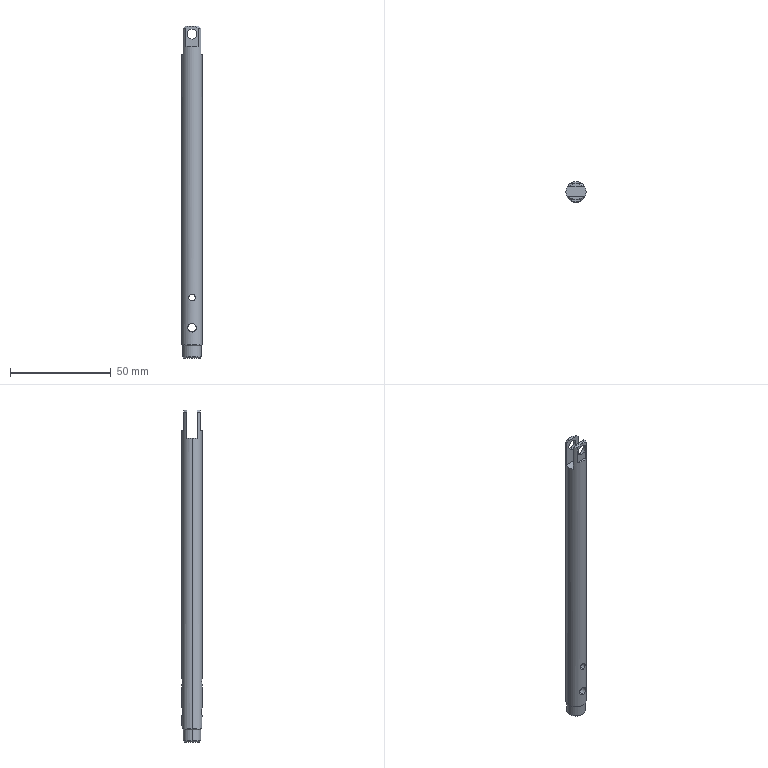Part | STEP file | PN_0103 Mount electronic clip sensor 1 | 1 solid | 30 faces | box 10 x 10 x 165 mm | volume 11828 mm3 | cylinder 12 | plane 10 | cone 8 | commonest cylinder face diameters 5 x4 3.3 x2 4.2 x2 9 x2 10 x2